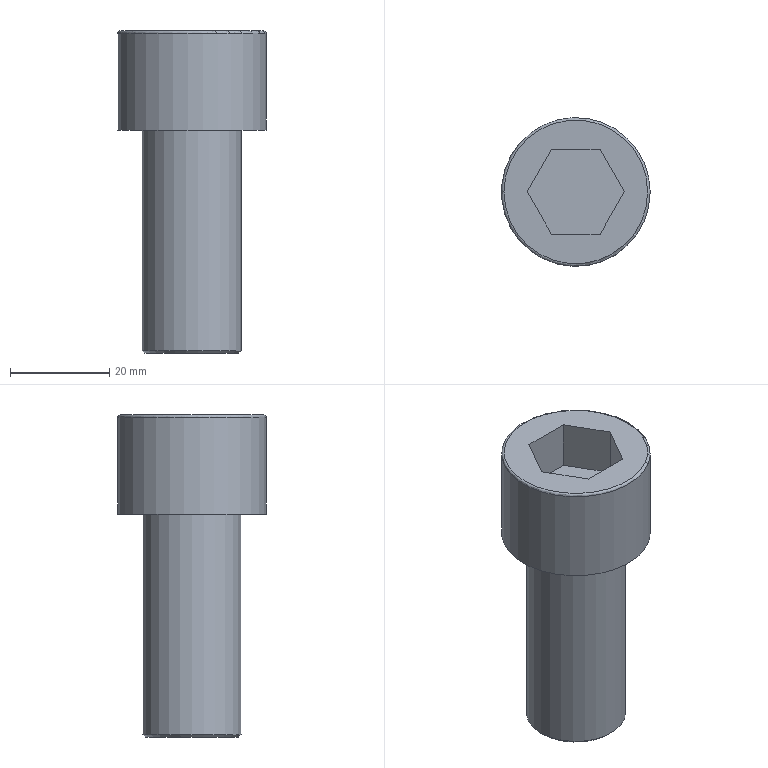Part | NX | features 模具.stp<1>[13] 2 | 1 solid | 14 faces | box 30 x 30 x 65 mm | volume 25759 mm3 | plane 10 | cylinder 2 | cone 1 | torus 1 | commonest cylinder face diameters 20 x1 30 x1
STEP:
#1=CARTESIAN_POINT('',(259.815,-225.,129.5));
#2=VERTEX_POINT('',#1);
#3=CARTESIAN_POINT('',(254.907,-216.5,129.5));
#4=VERTEX_POINT('',#3);
#5=CARTESIAN_POINT('',(259.815,-225.,129.5));
#6=DIRECTION('',(-0.5,0.866,0.));
#7=VECTOR('',#6,1000.);
#8=LINE('',#5,#7);
#9=EDGE_CURVE('',#2,#4,#8,.T.);
#10=ORIENTED_EDGE('',*,*,#9,.T.);
#11=CARTESIAN_POINT('',(245.093,-216.5,129.5));
#12=VERTEX_POINT('',#11);
#13=CARTESIAN_POINT('',(254.907,-216.5,129.5));
#14=DIRECTION('',(-1.,0.,0.));
#15=VECTOR('',#14,1000.);
#16=LINE('',#13,#15);
#17=EDGE_CURVE('',#4,#12,#16,.T.);
#18=ORIENTED_EDGE('',*,*,#17,.T.);
#19=CARTESIAN_POINT('',(240.185,-225.,129.5));
#20=VERTEX_POINT('',#19);
#21=CARTESIAN_POINT('',(245.093,-216.5,129.5));
#22=DIRECTION('',(-0.5,-0.866,0.));
#23=VECTOR('',#22,1000.);
#24=LINE('',#21,#23);
#25=EDGE_CURVE('',#12,#20,#24,.T.);
#26=ORIENTED_EDGE('',*,*,#25,.T.);
#27=CARTESIAN_POINT('',(245.093,-233.5,129.5));
#28=VERTEX_POINT('',#27);
#29=CARTESIAN_POINT('',(240.185,-225.,129.5));
#30=DIRECTION('',(0.5,-0.866,0.));
#31=VECTOR('',#30,1000.);
#32=LINE('',#29,#31);
#33=EDGE_CURVE('',#20,#28,#32,.T.);
#34=ORIENTED_EDGE('',*,*,#33,.T.);
#35=CARTESIAN_POINT('',(254.907,-233.5,129.5));
#36=VERTEX_POINT('',#35);
#37=CARTESIAN_POINT('',(245.093,-233.5,129.5));
#38=DIRECTION('',(1.,0.,0.));
#39=VECTOR('',#38,1000.);
#40=LINE('',#37,#39);
#41=EDGE_CURVE('',#28,#36,#40,.T.);
#42=ORIENTED_EDGE('',*,*,#41,.T.);
#43=CARTESIAN_POINT('',(254.907,-233.5,129.5));
#44=DIRECTION('',(0.5,0.866,0.));
#45=VECTOR('',#44,1000.);
#46=LINE('',#43,#45);
#47=EDGE_CURVE('',#36,#2,#46,.T.);
#48=ORIENTED_EDGE('',*,*,#47,.T.);
#49=EDGE_LOOP('',(#10,#18,#26,#34,#42,#48));
#50=FACE_BOUND('',#49,.T.);
#51=CARTESIAN_POINT('',(250.,-225.,129.5));
#52=DIRECTION('',(0.,0.,-1.));
#53=DIRECTION('',(0.,-1.,0.));
#54=AXIS2_PLACEMENT_3D('',#51,#52,#53);
#55=PLANE('',#54);
#56=ADVANCED_FACE('',(#50),#55,.F.);
#57=CARTESIAN_POINT('',(259.815,-225.,139.5));
#58=VERTEX_POINT('',#57);
#59=CARTESIAN_POINT('',(254.907,-216.5,139.5));
#60=VERTEX_POINT('',#59);
#61=CARTESIAN_POINT('',(259.815,-225.,139.5));
#62=DIRECTION('',(-0.5,0.866,0.));
#63=VECTOR('',#62,1000.);
#64=LINE('',#61,#63);
#65=EDGE_CURVE('',#58,#60,#64,.T.);
#66=ORIENTED_EDGE('',*,*,#65,.T.);
#67=CARTESIAN_POINT('',(254.907,-216.5,129.5));
#68=DIRECTION('',(0.,0.,1.));
#69=VECTOR('',#68,1000.);
#70=LINE('',#67,#69);
#71=EDGE_CURVE('',#4,#60,#70,.T.);
#72=ORIENTED_EDGE('',*,*,#71,.F.);
#73=ORIENTED_EDGE('',*,*,#9,.F.);
#74=CARTESIAN_POINT('',(259.815,-225.,129.5));
#75=DIRECTION('',(0.,0.,1.));
#76=VECTOR('',#75,1000.);
#77=LINE('',#74,#76);
#78=EDGE_CURVE('',#2,#58,#77,.T.);
#79=ORIENTED_EDGE('',*,*,#78,.T.);
#80=EDGE_LOOP('',(#66,#72,#73,#79));
#81=FACE_BOUND('',#80,.T.);
#82=CARTESIAN_POINT('',(257.361,-220.75,134.5));
#83=DIRECTION('',(0.866,0.5,0.));
#84=DIRECTION('',(0.,0.,-1.));
#85=AXIS2_PLACEMENT_3D('',#82,#83,#84);
#86=PLANE('',#85);
#87=ADVANCED_FACE('',(#81),#86,.F.);
#88=CARTESIAN_POINT('',(245.093,-216.5,139.5));
#89=VERTEX_POINT('',#88);
#90=CARTESIAN_POINT('',(254.907,-216.5,139.5));
#91=DIRECTION('',(-1.,0.,0.));
#92=VECTOR('',#91,1000.);
#93=LINE('',#90,#92);
#94=EDGE_CURVE('',#60,#89,#93,.T.);
#95=ORIENTED_EDGE('',*,*,#94,.T.);
#96=CARTESIAN_POINT('',(245.093,-216.5,129.5));
#97=DIRECTION('',(0.,0.,1.));
#98=VECTOR('',#97,1000.);
#99=LINE('',#96,#98);
#100=EDGE_CURVE('',#12,#89,#99,.T.);
#101=ORIENTED_EDGE('',*,*,#100,.F.);
#102=ORIENTED_EDGE('',*,*,#17,.F.);
#103=ORIENTED_EDGE('',*,*,#71,.T.);
#104=EDGE_LOOP('',(#95,#101,#102,#103));
#105=FACE_BOUND('',#104,.T.);
#106=CARTESIAN_POINT('',(250.,-216.5,134.5));
#107=DIRECTION('',(0.,1.,0.));
#108=DIRECTION('',(0.,0.,-1.));
#109=AXIS2_PLACEMENT_3D('',#106,#107,#108);
#110=PLANE('',#109);
#111=ADVANCED_FACE('',(#105),#110,.F.);
#112=CARTESIAN_POINT('',(240.185,-225.,139.5));
#113=VERTEX_POINT('',#112);
#114=CARTESIAN_POINT('',(245.093,-216.5,139.5));
#115=DIRECTION('',(-0.5,-0.866,0.));
#116=VECTOR('',#115,1000.);
#117=LINE('',#114,#116);
#118=EDGE_CURVE('',#89,#113,#117,.T.);
#119=ORIENTED_EDGE('',*,*,#118,.T.);
#120=CARTESIAN_POINT('',(240.185,-225.,129.5));
#121=DIRECTION('',(0.,0.,1.));
#122=VECTOR('',#121,1000.);
#123=LINE('',#120,#122);
#124=EDGE_CURVE('',#20,#113,#123,.T.);
#125=ORIENTED_EDGE('',*,*,#124,.F.);
#126=ORIENTED_EDGE('',*,*,#25,.F.);
#127=ORIENTED_EDGE('',*,*,#100,.T.);
#128=EDGE_LOOP('',(#119,#125,#126,#127));
#129=FACE_BOUND('',#128,.T.);
#130=CARTESIAN_POINT('',(242.639,-220.75,134.5));
#131=DIRECTION('',(-0.866,0.5,0.));
#132=DIRECTION('',(0.,0.,1.));
#133=AXIS2_PLACEMENT_3D('',#130,#131,#132);
#134=PLANE('',#133);
#135=ADVANCED_FACE('',(#129),#134,.F.);
#136=CARTESIAN_POINT('',(245.093,-233.5,139.5));
#137=VERTEX_POINT('',#136);
#138=CARTESIAN_POINT('',(240.185,-225.,139.5));
#139=DIRECTION('',(0.5,-0.866,0.));
#140=VECTOR('',#139,1000.);
#141=LINE('',#138,#140);
#142=EDGE_CURVE('',#113,#137,#141,.T.);
#143=ORIENTED_EDGE('',*,*,#142,.T.);
#144=CARTESIAN_POINT('',(245.093,-233.5,129.5));
#145=DIRECTION('',(0.,0.,1.));
#146=VECTOR('',#145,1000.);
#147=LINE('',#144,#146);
#148=EDGE_CURVE('',#28,#137,#147,.T.);
#149=ORIENTED_EDGE('',*,*,#148,.F.);
#150=ORIENTED_EDGE('',*,*,#33,.F.);
#151=ORIENTED_EDGE('',*,*,#124,.T.);
#152=EDGE_LOOP('',(#143,#149,#150,#151));
#153=FACE_BOUND('',#152,.T.);
#154=CARTESIAN_POINT('',(242.639,-229.25,134.5));
#155=DIRECTION('',(-0.866,-0.5,0.));
#156=DIRECTION('',(-0.5,0.866,0.));
#157=AXIS2_PLACEMENT_3D('',#154,#155,#156);
#158=PLANE('',#157);
#159=ADVANCED_FACE('',(#153),#158,.F.);
#160=CARTESIAN_POINT('',(254.907,-233.5,139.5));
#161=VERTEX_POINT('',#160);
#162=CARTESIAN_POINT('',(245.093,-233.5,139.5));
#163=DIRECTION('',(1.,0.,0.));
#164=VECTOR('',#163,1000.);
#165=LINE('',#162,#164);
#166=EDGE_CURVE('',#137,#161,#165,.T.);
#167=ORIENTED_EDGE('',*,*,#166,.T.);
#168=CARTESIAN_POINT('',(254.907,-233.5,129.5));
#169=DIRECTION('',(0.,0.,1.));
#170=VECTOR('',#169,1000.);
#171=LINE('',#168,#170);
#172=EDGE_CURVE('',#36,#161,#171,.T.);
#173=ORIENTED_EDGE('',*,*,#172,.F.);
#174=ORIENTED_EDGE('',*,*,#41,.F.);
#175=ORIENTED_EDGE('',*,*,#148,.T.);
#176=EDGE_LOOP('',(#167,#173,#174,#175));
#177=FACE_BOUND('',#176,.T.);
#178=CARTESIAN_POINT('',(250.,-233.5,134.5));
#179=DIRECTION('',(0.,-1.,0.));
#180=DIRECTION('',(-1.,0.,0.));
#181=AXIS2_PLACEMENT_3D('',#178,#179,#180);
#182=PLANE('',#181);
#183=ADVANCED_FACE('',(#177),#182,.F.);
#184=CARTESIAN_POINT('',(254.907,-233.5,139.5));
#185=DIRECTION('',(0.5,0.866,0.));
#186=VECTOR('',#185,1000.);
#187=LINE('',#184,#186);
#188=EDGE_CURVE('',#161,#58,#187,.T.);
#189=ORIENTED_EDGE('',*,*,#188,.T.);
#190=ORIENTED_EDGE('',*,*,#78,.F.);
#191=ORIENTED_EDGE('',*,*,#47,.F.);
#192=ORIENTED_EDGE('',*,*,#172,.T.);
#193=EDGE_LOOP('',(#189,#190,#191,#192));
#194=FACE_BOUND('',#193,.T.);
#195=CARTESIAN_POINT('',(257.361,-229.25,134.5));
#196=DIRECTION('',(0.866,-0.5,0.));
#197=DIRECTION('',(0.,0.,-1.));
#198=AXIS2_PLACEMENT_3D('',#195,#196,#197);
#199=PLANE('',#198);
#200=ADVANCED_FACE('',(#194),#199,.F.);
#201=CARTESIAN_POINT('',(240.,-225.,75.));
#202=VERTEX_POINT('',#201);
#203=CARTESIAN_POINT('',(250.,-225.,75.));
#204=DIRECTION('',(0.,0.,1.));
#205=DIRECTION('',(-1.,0.,0.));
#206=AXIS2_PLACEMENT_3D('',#203,#204,#205);
#207=CIRCLE('',#206,10.);
#208=EDGE_CURVE('',#202,#202,#207,.T.);
#209=ORIENTED_EDGE('',*,*,#208,.F.);
#210=EDGE_LOOP('',(#209));
#211=FACE_BOUND('',#210,.T.);
#212=CARTESIAN_POINT('',(240.5,-225.,74.5));
#213=VERTEX_POINT('',#212);
#214=CARTESIAN_POINT('',(250.,-225.,74.5));
#215=DIRECTION('',(0.,0.,-1.));
#216=DIRECTION('',(-1.,0.,0.));
#217=AXIS2_PLACEMENT_3D('',#214,#215,#216);
#218=CIRCLE('',#217,9.5);
#219=EDGE_CURVE('',#213,#213,#218,.T.);
#220=ORIENTED_EDGE('',*,*,#219,.F.);
#221=EDGE_LOOP('',(#220));
#222=FACE_BOUND('',#221,.T.);
#223=CARTESIAN_POINT('',(250.,-225.,75.));
#224=DIRECTION('',(0.,0.,1.));
#225=DIRECTION('',(1.,0.,0.));
#226=AXIS2_PLACEMENT_3D('',#223,#224,#225);
#227=CONICAL_SURFACE('',#226,10.,0.7854);
#228=ADVANCED_FACE('',(#211,#222),#227,.T.);
#229=CARTESIAN_POINT('',(260.,-225.,119.5));
#230=VERTEX_POINT('',#229);
#231=CARTESIAN_POINT('',(250.,-225.,119.5));
#232=DIRECTION('',(0.,0.,-1.));
#233=DIRECTION('',(1.,0.,0.));
#234=AXIS2_PLACEMENT_3D('',#231,#232,#233);
#235=CIRCLE('',#234,10.);
#236=EDGE_CURVE('',#230,#230,#235,.T.);
#237=ORIENTED_EDGE('',*,*,#236,.T.);
#238=EDGE_LOOP('',(#237));
#239=FACE_BOUND('',#238,.T.);
#240=ORIENTED_EDGE('',*,*,#208,.T.);
#241=EDGE_LOOP('',(#240));
#242=FACE_BOUND('',#241,.T.);
#243=CARTESIAN_POINT('',(250.,-225.,74.5));
#244=DIRECTION('',(0.,0.,1.));
#245=DIRECTION('',(1.,0.,0.));
#246=AXIS2_PLACEMENT_3D('',#243,#244,#245);
#247=CYLINDRICAL_SURFACE('',#246,10.);
#248=ADVANCED_FACE('',(#239,#242),#247,.T.);
#249=ORIENTED_EDGE('',*,*,#219,.T.);
#250=EDGE_LOOP('',(#249));
#251=FACE_BOUND('',#250,.T.);
#252=CARTESIAN_POINT('',(250.,-225.,74.5));
#253=DIRECTION('',(0.,0.,-1.));
#254=DIRECTION('',(0.,-1.,0.));
#255=AXIS2_PLACEMENT_3D('',#252,#253,#254);
#256=PLANE('',#255);
#257=ADVANCED_FACE('',(#251),#256,.T.);
#258=CARTESIAN_POINT('',(265.,-225.,139.));
#259=VERTEX_POINT('',#258);
#260=CARTESIAN_POINT('',(250.,-225.,139.));
#261=DIRECTION('',(0.,0.,-1.));
#262=DIRECTION('',(1.,0.,0.));
#263=AXIS2_PLACEMENT_3D('',#260,#261,#262);
#264=CIRCLE('',#263,15.);
#265=EDGE_CURVE('',#259,#259,#264,.T.);
#266=ORIENTED_EDGE('',*,*,#265,.F.);
#267=EDGE_LOOP('',(#266));
#268=FACE_BOUND('',#267,.T.);
#269=CARTESIAN_POINT('',(264.5,-225.,139.5));
#270=VERTEX_POINT('',#269);
#271=CARTESIAN_POINT('',(250.,-225.,139.5));
#272=DIRECTION('',(0.,0.,1.));
#273=DIRECTION('',(1.,0.,0.));
#274=AXIS2_PLACEMENT_3D('',#271,#272,#273);
#275=CIRCLE('',#274,14.5);
#276=EDGE_CURVE('',#270,#270,#275,.T.);
#277=ORIENTED_EDGE('',*,*,#276,.F.);
#278=EDGE_LOOP('',(#277));
#279=FACE_BOUND('',#278,.T.);
#280=CARTESIAN_POINT('',(250.,-225.,139.));
#281=DIRECTION('',(0.,0.,1.));
#282=DIRECTION('',(1.,0.,0.));
#283=AXIS2_PLACEMENT_3D('',#280,#281,#282);
#284=TOROIDAL_SURFACE('',#283,14.5,0.5);
#285=ADVANCED_FACE('',(#268,#279),#284,.T.);
#286=CARTESIAN_POINT('',(265.,-225.,119.5));
#287=VERTEX_POINT('',#286);
#288=CARTESIAN_POINT('',(250.,-225.,119.5));
#289=DIRECTION('',(0.,0.,1.));
#290=DIRECTION('',(1.,0.,0.));
#291=AXIS2_PLACEMENT_3D('',#288,#289,#290);
#292=CIRCLE('',#291,15.);
#293=EDGE_CURVE('',#287,#287,#292,.T.);
#294=ORIENTED_EDGE('',*,*,#293,.T.);
#295=EDGE_LOOP('',(#294));
#296=FACE_BOUND('',#295,.T.);
#297=ORIENTED_EDGE('',*,*,#265,.T.);
#298=EDGE_LOOP('',(#297));
#299=FACE_BOUND('',#298,.T.);
#300=CARTESIAN_POINT('',(250.,-225.,119.5));
#301=DIRECTION('',(0.,0.,1.));
#302=DIRECTION('',(1.,0.,0.));
#303=AXIS2_PLACEMENT_3D('',#300,#301,#302);
#304=CYLINDRICAL_SURFACE('',#303,15.);
#305=ADVANCED_FACE('',(#296,#299),#304,.T.);
#306=ORIENTED_EDGE('',*,*,#293,.F.);
#307=EDGE_LOOP('',(#306));
#308=FACE_BOUND('',#307,.T.);
#309=ORIENTED_EDGE('',*,*,#236,.F.);
#310=EDGE_LOOP('',(#309));
#311=FACE_BOUND('',#310,.T.);
#312=CARTESIAN_POINT('',(250.,-225.,119.5));
#313=DIRECTION('',(0.,0.,-1.));
#314=DIRECTION('',(0.,-1.,0.));
#315=AXIS2_PLACEMENT_3D('',#312,#313,#314);
#316=PLANE('',#315);
#317=ADVANCED_FACE('',(#308,#311),#316,.T.);
#318=ORIENTED_EDGE('',*,*,#276,.T.);
#319=EDGE_LOOP('',(#318));
#320=FACE_BOUND('',#319,.T.);
#321=ORIENTED_EDGE('',*,*,#188,.F.);
#322=ORIENTED_EDGE('',*,*,#166,.F.);
#323=ORIENTED_EDGE('',*,*,#142,.F.);
#324=ORIENTED_EDGE('',*,*,#118,.F.);
#325=ORIENTED_EDGE('',*,*,#94,.F.);
#326=ORIENTED_EDGE('',*,*,#65,.F.);
#327=EDGE_LOOP('',(#321,#322,#323,#324,#325,#326));
#328=FACE_BOUND('',#327,.T.);
#329=CARTESIAN_POINT('',(250.,-225.,139.5));
#330=DIRECTION('',(0.,0.,1.));
#331=DIRECTION('',(1.,0.,0.));
#332=AXIS2_PLACEMENT_3D('',#329,#330,#331);
#333=PLANE('',#332);
#334=ADVANCED_FACE('',(#320,#328),#333,.T.);
#335=CLOSED_SHELL('',(#56,#87,#111,#135,#159,#183,#200,#228,#248,#257,#285,#305,#317,#334));
#336=MANIFOLD_SOLID_BREP('',#335);
#337=(LENGTH_UNIT()NAMED_UNIT(*)SI_UNIT(.MILLI.,.METRE.));
#338=UNCERTAINTY_MEASURE_WITH_UNIT(LENGTH_MEASURE(0.00001),#337,'','');
#339=(NAMED_UNIT(*)PLANE_ANGLE_UNIT()SI_UNIT($,.RADIAN.));
#340=(NAMED_UNIT(*)SI_UNIT($,.STERADIAN.)SOLID_ANGLE_UNIT());
#341=(GEOMETRIC_REPRESENTATION_CONTEXT(3)GLOBAL_UNCERTAINTY_ASSIGNED_CONTEXT((#338))GLOBAL_UNIT_ASSIGNED_CONTEXT((#337,#339,#340))REPRESENTATION_CONTEXT('',''));
#342=ADVANCED_BREP_SHAPE_REPRESENTATION('',(#336),#341);